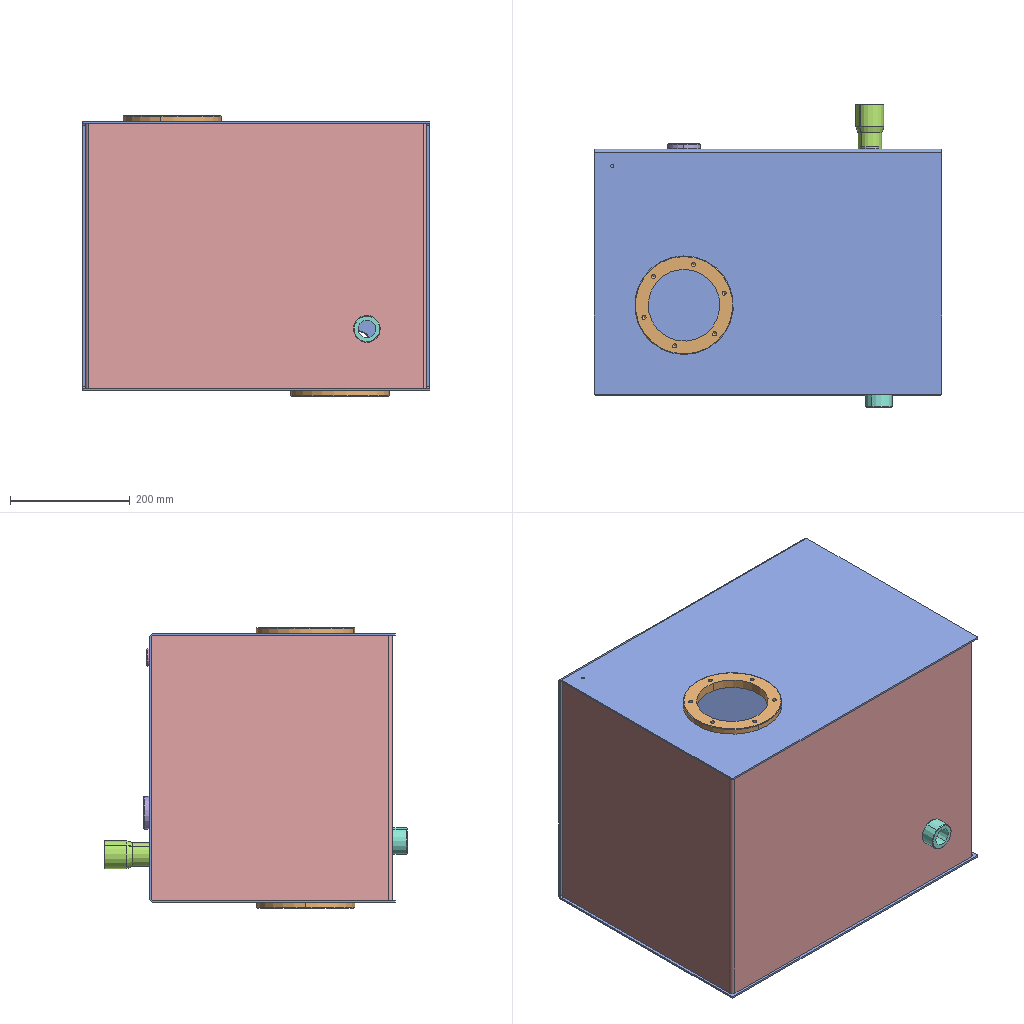Assembly | SolidWorks | 7 different items | 8 placed | box 581 x 506 x 470 mm
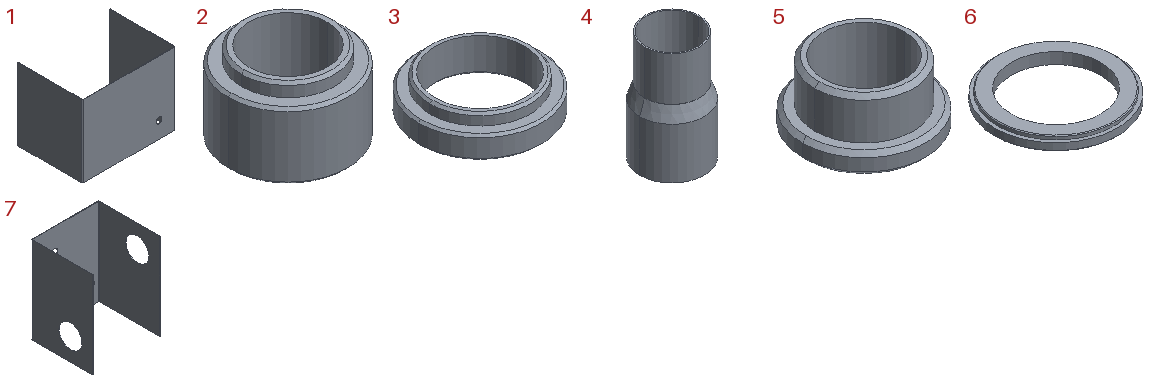Parts list (item | quantity | size | volume | features):
1 | x1 | 571 x 403 x 444 mm | 1818117 mm3 | features ICE 2, FlatPattern 1, SMBaseFlange 1, SheetMetal 1
2 | x1 | 45 x 45 x 30 mm | 23873 mm3 | features Chamfer 1, Extrusion 1, ICE 1
3 | x1 | 55 x 55 x 15 mm | 12557 mm3 | features Chamfer 1, Extrusion 1, ICE 1
4 | x1 | 47 x 47 x 79 mm | 10172 mm3 | features 3DProfileFeature 2, ICE 2, NetBlend 1, NetBlendCut 1
5 | x1 | 30 x 30 x 15 mm | 3311 mm3 | features Chamfer 1, Extrusion 1, ICE 1
6 | x2 | 165 x 165 x 15 mm | 136481 mm3 | features 3DProfileFeature 1, Chamfer 1, Extrusion 1, HoleWzd 1, ICE 1
7 | x1 | 450 x 411 x 581 mm | 2075079 mm3 | features ICE 4, FlatPattern 1, SMBaseFlange 1, SheetMetal 1
Mates (type | each side: item.copy, entity, surface, feature):
Coincident | 1.1 face plane Base-Flange1 | 7.1 face plane Base-Flange1 | 2 times
DistanceDim | 7.1 face plane Base-Flange1 | 1.1 face plane Base-Flange1
Concentric | 7.1 edge | 4.1 edge
DistanceDim | 4.1 face plane Boss-Extrude1 | 7.1 face plane Base-Flange1
Coincident | 7.1 face plane Base-Flange1 | 5.1 face plane Boss-Extrude1
Concentric | 7.1 edge | 5.1 edge
Coincident | 7.1 face plane Base-Flange1 | 6.1 face plane Boss-Extrude1
Concentric | 7.1 edge | 6.1 edge
Coincident | 7.1 face plane Base-Flange1 | 6.2 face plane Boss-Extrude1
Concentric | 7.1 edge | 6.2 edge
Coincident | 1.1 face plane Base-Flange1 | 2.1 face plane Boss-Extrude1
Concentric | 1.1 edge | 2.1 edge
Coincident | 7.1 face plane Base-Flange1 | 3.1 face plane Cut-Extrude1
Concentric | 7.1 edge | 3.1 edge